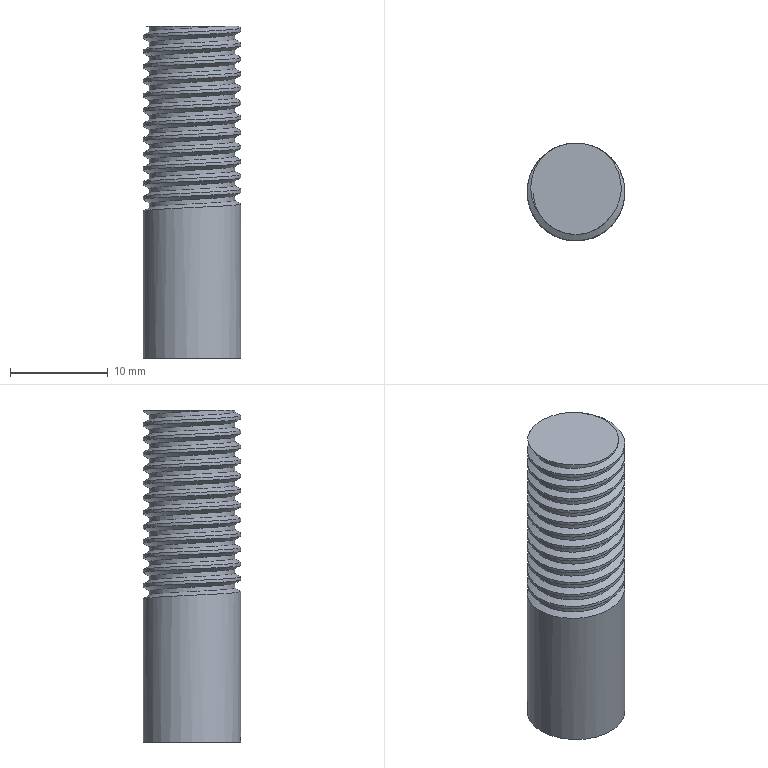Part | NX | features solid 2 | 1 solid | 19 faces | box 10 x 10 x 34 mm | volume 2528 mm3 | cylinder 14 | plane 3 | spline 2 | commonest cylinder face diameters 10 x13 8.75 x1